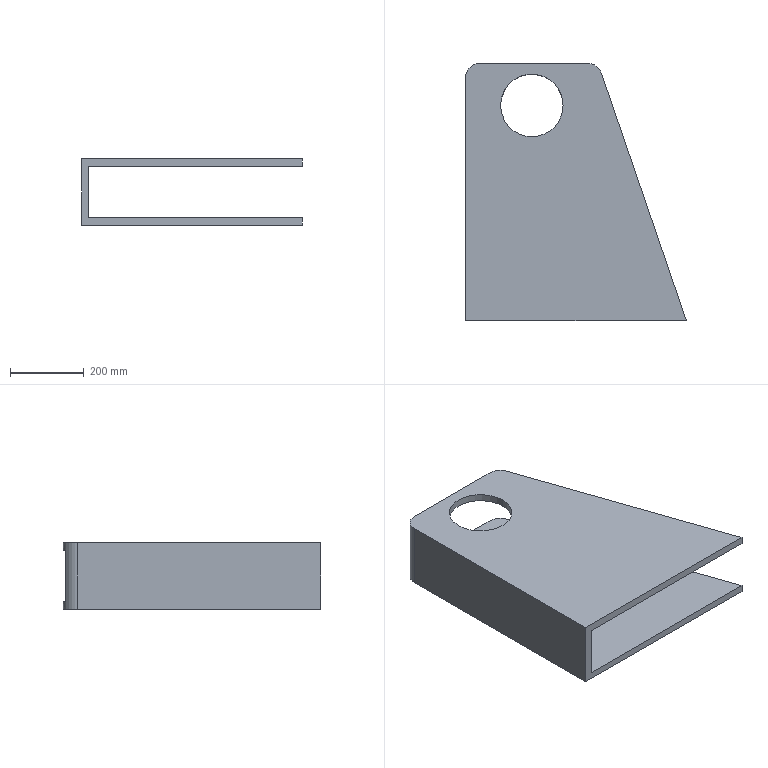Part | SolidWorks | features ICE 3, Fillet 2, Extrusion 1 | 1 solid | 18 faces | box 600 x 700 x 180 mm | volume 14429116 mm3 | plane 11 | cylinder 7 | commonest cylinder face diameters 170 x4 80 x3
STEP:
#1=CARTESIAN_POINT('',(95.,585.,-20.));
#2=VERTEX_POINT('',#1);
#3=CARTESIAN_POINT('',(265.,585.,-20.));
#4=VERTEX_POINT('',#3);
#5=CARTESIAN_POINT('',(180.,585.,-20.));
#6=DIRECTION('',(0.,0.,1.));
#7=DIRECTION('',(1.,0.,0.));
#8=AXIS2_PLACEMENT_3D('',#5,#6,#7);
#9=CIRCLE('',#8,85.);
#10=EDGE_CURVE('',#2,#4,#9,.T.);
#11=ORIENTED_EDGE('',*,*,#10,.F.);
#12=CARTESIAN_POINT('',(95.,585.,0.));
#13=VERTEX_POINT('',#12);
#14=CARTESIAN_POINT('',(95.,585.,-190.));
#15=DIRECTION('',(0.,0.,1.));
#16=VECTOR('',#15,1000.);
#17=LINE('',#14,#16);
#18=EDGE_CURVE('',#2,#13,#17,.T.);
#19=ORIENTED_EDGE('',*,*,#18,.T.);
#20=CARTESIAN_POINT('',(265.,585.,0.));
#21=VERTEX_POINT('',#20);
#22=CARTESIAN_POINT('',(180.,585.,0.));
#23=DIRECTION('',(0.,0.,1.));
#24=DIRECTION('',(1.,0.,0.));
#25=AXIS2_PLACEMENT_3D('',#22,#23,#24);
#26=CIRCLE('',#25,85.);
#27=EDGE_CURVE('',#13,#21,#26,.T.);
#28=ORIENTED_EDGE('',*,*,#27,.T.);
#29=CARTESIAN_POINT('',(265.,585.,-190.));
#30=DIRECTION('',(0.,0.,1.));
#31=VECTOR('',#30,1000.);
#32=LINE('',#29,#31);
#33=EDGE_CURVE('',#4,#21,#32,.T.);
#34=ORIENTED_EDGE('',*,*,#33,.F.);
#35=EDGE_LOOP('',(#11,#19,#28,#34));
#36=FACE_OUTER_BOUND('',#35,.T.);
#37=CARTESIAN_POINT('',(180.,585.,-190.));
#38=DIRECTION('',(0.,0.,1.));
#39=DIRECTION('',(1.,0.,0.));
#40=AXIS2_PLACEMENT_3D('',#37,#38,#39);
#41=CYLINDRICAL_SURFACE('',#40,85.);
#42=ADVANCED_FACE('',(#36),#41,.F.);
#43=CARTESIAN_POINT('',(95.,585.,-180.));
#44=VERTEX_POINT('',#43);
#45=CARTESIAN_POINT('',(265.,585.,-180.));
#46=VERTEX_POINT('',#45);
#47=CARTESIAN_POINT('',(180.,585.,-180.));
#48=DIRECTION('',(0.,0.,1.));
#49=DIRECTION('',(1.,0.,0.));
#50=AXIS2_PLACEMENT_3D('',#47,#48,#49);
#51=CIRCLE('',#50,85.);
#52=EDGE_CURVE('',#44,#46,#51,.T.);
#53=ORIENTED_EDGE('',*,*,#52,.F.);
#54=CARTESIAN_POINT('',(95.,585.,-160.));
#55=VERTEX_POINT('',#54);
#56=CARTESIAN_POINT('',(95.,585.,-190.));
#57=DIRECTION('',(0.,0.,1.));
#58=VECTOR('',#57,1000.);
#59=LINE('',#56,#58);
#60=EDGE_CURVE('',#44,#55,#59,.T.);
#61=ORIENTED_EDGE('',*,*,#60,.T.);
#62=CARTESIAN_POINT('',(265.,585.,-160.));
#63=VERTEX_POINT('',#62);
#64=CARTESIAN_POINT('',(180.,585.,-160.));
#65=DIRECTION('',(0.,0.,-1.));
#66=DIRECTION('',(-1.,0.,0.));
#67=AXIS2_PLACEMENT_3D('',#64,#65,#66);
#68=CIRCLE('',#67,85.);
#69=EDGE_CURVE('',#63,#55,#68,.T.);
#70=ORIENTED_EDGE('',*,*,#69,.F.);
#71=CARTESIAN_POINT('',(265.,585.,-190.));
#72=DIRECTION('',(0.,0.,1.));
#73=VECTOR('',#72,1000.);
#74=LINE('',#71,#73);
#75=EDGE_CURVE('',#46,#63,#74,.T.);
#76=ORIENTED_EDGE('',*,*,#75,.F.);
#77=EDGE_LOOP('',(#53,#61,#70,#76));
#78=FACE_OUTER_BOUND('',#77,.T.);
#79=CARTESIAN_POINT('',(180.,585.,-190.));
#80=DIRECTION('',(0.,0.,1.));
#81=DIRECTION('',(1.,0.,0.));
#82=AXIS2_PLACEMENT_3D('',#79,#80,#81);
#83=CYLINDRICAL_SURFACE('',#82,85.);
#84=ADVANCED_FACE('',(#78),#83,.F.);
#85=CARTESIAN_POINT('',(331.429,700.,-180.));
#86=VERTEX_POINT('',#85);
#87=CARTESIAN_POINT('',(40.,700.,-180.));
#88=VERTEX_POINT('',#87);
#89=CARTESIAN_POINT('',(0.,700.,-180.));
#90=DIRECTION('',(-1.,0.,0.));
#91=VECTOR('',#90,1000.);
#92=LINE('',#89,#91);
#93=EDGE_CURVE('',#86,#88,#92,.T.);
#94=ORIENTED_EDGE('',*,*,#93,.T.);
#95=CARTESIAN_POINT('',(40.,700.,-160.));
#96=VERTEX_POINT('',#95);
#97=CARTESIAN_POINT('',(40.,700.,0.));
#98=DIRECTION('',(0.,0.,1.));
#99=VECTOR('',#98,1000.);
#100=LINE('',#97,#99);
#101=EDGE_CURVE('',#88,#96,#100,.T.);
#102=ORIENTED_EDGE('',*,*,#101,.T.);
#103=CARTESIAN_POINT('',(331.429,700.,-160.));
#104=VERTEX_POINT('',#103);
#105=CARTESIAN_POINT('',(360.,700.,-160.));
#106=DIRECTION('',(1.,0.,0.));
#107=VECTOR('',#106,1000.);
#108=LINE('',#105,#107);
#109=EDGE_CURVE('',#96,#104,#108,.T.);
#110=ORIENTED_EDGE('',*,*,#109,.T.);
#111=CARTESIAN_POINT('',(331.429,700.,-180.));
#112=DIRECTION('',(0.,0.,-1.));
#113=VECTOR('',#112,1000.);
#114=LINE('',#111,#113);
#115=EDGE_CURVE('',#104,#86,#114,.T.);
#116=ORIENTED_EDGE('',*,*,#115,.T.);
#117=EDGE_LOOP('',(#94,#102,#110,#116));
#118=FACE_OUTER_BOUND('',#117,.T.);
#119=CARTESIAN_POINT('',(0.,700.,0.));
#120=DIRECTION('',(0.,-1.,0.));
#121=DIRECTION('',(0.,0.,-1.));
#122=AXIS2_PLACEMENT_3D('',#119,#120,#121);
#123=PLANE('',#122);
#124=ADVANCED_FACE('',(#118),#123,.F.);
#125=CARTESIAN_POINT('',(180.,585.,0.));
#126=DIRECTION('',(0.,0.,1.));
#127=DIRECTION('',(1.,0.,0.));
#128=AXIS2_PLACEMENT_3D('',#125,#126,#127);
#129=CIRCLE('',#128,85.);
#130=EDGE_CURVE('',#21,#13,#129,.T.);
#131=ORIENTED_EDGE('',*,*,#130,.F.);
#132=ORIENTED_EDGE('',*,*,#27,.F.);
#133=EDGE_LOOP('',(#131,#132));
#134=FACE_BOUND('',#133,.T.);
#135=CARTESIAN_POINT('',(40.,700.,0.));
#136=VERTEX_POINT('',#135);
#137=CARTESIAN_POINT('',(331.429,700.,0.));
#138=VERTEX_POINT('',#137);
#139=CARTESIAN_POINT('',(360.,700.,0.));
#140=DIRECTION('',(1.,0.,0.));
#141=VECTOR('',#140,1000.);
#142=LINE('',#139,#141);
#143=EDGE_CURVE('',#136,#138,#142,.T.);
#144=ORIENTED_EDGE('',*,*,#143,.F.);
#145=CARTESIAN_POINT('',(0.,660.,0.));
#146=VERTEX_POINT('',#145);
#147=CARTESIAN_POINT('',(40.,660.,0.));
#148=DIRECTION('',(0.,0.,1.));
#149=DIRECTION('',(-1.,0.,0.));
#150=AXIS2_PLACEMENT_3D('',#147,#148,#149);
#151=CIRCLE('',#150,40.);
#152=EDGE_CURVE('',#136,#146,#151,.T.);
#153=ORIENTED_EDGE('',*,*,#152,.T.);
#154=CARTESIAN_POINT('',(0.,0.,0.));
#155=VERTEX_POINT('',#154);
#156=CARTESIAN_POINT('',(0.,700.,0.));
#157=DIRECTION('',(0.,-1.,0.));
#158=VECTOR('',#157,1000.);
#159=LINE('',#156,#158);
#160=EDGE_CURVE('',#146,#155,#159,.T.);
#161=ORIENTED_EDGE('',*,*,#160,.T.);
#162=CARTESIAN_POINT('',(600.,0.,0.));
#163=VERTEX_POINT('',#162);
#164=CARTESIAN_POINT('',(360.,0.,0.));
#165=DIRECTION('',(1.,0.,0.));
#166=VECTOR('',#165,1000.);
#167=LINE('',#164,#166);
#168=EDGE_CURVE('',#155,#163,#167,.T.);
#169=ORIENTED_EDGE('',*,*,#168,.T.);
#170=CARTESIAN_POINT('',(369.266,672.973,0.));
#171=VERTEX_POINT('',#170);
#172=CARTESIAN_POINT('',(360.,700.,0.));
#173=DIRECTION('',(-0.3243,0.9459,0.));
#174=VECTOR('',#173,1000.);
#175=LINE('',#172,#174);
#176=EDGE_CURVE('',#163,#171,#175,.T.);
#177=ORIENTED_EDGE('',*,*,#176,.T.);
#178=CARTESIAN_POINT('',(331.429,660.,0.));
#179=DIRECTION('',(0.,0.,1.));
#180=DIRECTION('',(-1.,0.,0.));
#181=AXIS2_PLACEMENT_3D('',#178,#179,#180);
#182=CIRCLE('',#181,40.);
#183=EDGE_CURVE('',#171,#138,#182,.T.);
#184=ORIENTED_EDGE('',*,*,#183,.T.);
#185=EDGE_LOOP('',(#144,#153,#161,#169,#177,#184));
#186=FACE_OUTER_BOUND('',#185,.T.);
#187=CARTESIAN_POINT('',(360.,700.,0.));
#188=DIRECTION('',(0.,0.,-1.));
#189=DIRECTION('',(-1.,0.,0.));
#190=AXIS2_PLACEMENT_3D('',#187,#188,#189);
#191=PLANE('',#190);
#192=ADVANCED_FACE('',(#134,#186),#191,.F.);
#193=CARTESIAN_POINT('',(180.,585.,-20.));
#194=DIRECTION('',(0.,0.,1.));
#195=DIRECTION('',(1.,0.,0.));
#196=AXIS2_PLACEMENT_3D('',#193,#194,#195);
#197=CIRCLE('',#196,85.);
#198=EDGE_CURVE('',#4,#2,#197,.T.);
#199=ORIENTED_EDGE('',*,*,#198,.T.);
#200=ORIENTED_EDGE('',*,*,#10,.T.);
#201=EDGE_LOOP('',(#199,#200));
#202=FACE_BOUND('',#201,.T.);
#203=CARTESIAN_POINT('',(20.,694.641,-20.));
#204=VERTEX_POINT('',#203);
#205=CARTESIAN_POINT('',(20.,0.,-20.));
#206=VERTEX_POINT('',#205);
#207=CARTESIAN_POINT('',(20.,700.,-20.));
#208=DIRECTION('',(0.,-1.,0.));
#209=VECTOR('',#208,1000.);
#210=LINE('',#207,#209);
#211=EDGE_CURVE('',#204,#206,#210,.T.);
#212=ORIENTED_EDGE('',*,*,#211,.F.);
#213=CARTESIAN_POINT('',(40.,700.,-20.));
#214=VERTEX_POINT('',#213);
#215=CARTESIAN_POINT('',(40.,660.,-20.));
#216=DIRECTION('',(0.,0.,-1.));
#217=DIRECTION('',(1.,0.,0.));
#218=AXIS2_PLACEMENT_3D('',#215,#216,#217);
#219=CIRCLE('',#218,40.);
#220=EDGE_CURVE('',#204,#214,#219,.T.);
#221=ORIENTED_EDGE('',*,*,#220,.T.);
#222=CARTESIAN_POINT('',(331.429,700.,-20.));
#223=VERTEX_POINT('',#222);
#224=CARTESIAN_POINT('',(20.,700.,-20.));
#225=DIRECTION('',(-1.,0.,0.));
#226=VECTOR('',#225,1000.);
#227=LINE('',#224,#226);
#228=EDGE_CURVE('',#223,#214,#227,.T.);
#229=ORIENTED_EDGE('',*,*,#228,.F.);
#230=CARTESIAN_POINT('',(369.266,672.973,-20.));
#231=VERTEX_POINT('',#230);
#232=CARTESIAN_POINT('',(331.429,660.,-20.));
#233=DIRECTION('',(0.,0.,-1.));
#234=DIRECTION('',(1.,0.,0.));
#235=AXIS2_PLACEMENT_3D('',#232,#233,#234);
#236=CIRCLE('',#235,40.);
#237=EDGE_CURVE('',#223,#231,#236,.T.);
#238=ORIENTED_EDGE('',*,*,#237,.T.);
#239=CARTESIAN_POINT('',(600.,0.,-20.));
#240=VERTEX_POINT('',#239);
#241=CARTESIAN_POINT('',(360.,700.,-20.));
#242=DIRECTION('',(-0.3243,0.9459,0.));
#243=VECTOR('',#242,1000.);
#244=LINE('',#241,#243);
#245=EDGE_CURVE('',#240,#231,#244,.T.);
#246=ORIENTED_EDGE('',*,*,#245,.F.);
#247=CARTESIAN_POINT('',(20.,0.,-20.));
#248=DIRECTION('',(-1.,0.,0.));
#249=VECTOR('',#248,1000.);
#250=LINE('',#247,#249);
#251=EDGE_CURVE('',#240,#206,#250,.T.);
#252=ORIENTED_EDGE('',*,*,#251,.T.);
#253=EDGE_LOOP('',(#212,#221,#229,#238,#246,#252));
#254=FACE_OUTER_BOUND('',#253,.T.);
#255=CARTESIAN_POINT('',(20.,700.,-20.));
#256=DIRECTION('',(0.,0.,1.));
#257=DIRECTION('',(1.,0.,0.));
#258=AXIS2_PLACEMENT_3D('',#255,#256,#257);
#259=PLANE('',#258);
#260=ADVANCED_FACE('',(#202,#254),#259,.F.);
#261=CARTESIAN_POINT('',(20.,694.641,-160.));
#262=VERTEX_POINT('',#261);
#263=CARTESIAN_POINT('',(20.,0.,-160.));
#264=VERTEX_POINT('',#263);
#265=CARTESIAN_POINT('',(20.,700.,-160.));
#266=DIRECTION('',(0.,-1.,0.));
#267=VECTOR('',#266,1000.);
#268=LINE('',#265,#267);
#269=EDGE_CURVE('',#262,#264,#268,.T.);
#270=ORIENTED_EDGE('',*,*,#269,.F.);
#271=CARTESIAN_POINT('',(20.,694.641,-160.));
#272=DIRECTION('',(0.,0.,1.));
#273=VECTOR('',#272,1000.);
#274=LINE('',#271,#273);
#275=EDGE_CURVE('',#262,#204,#274,.T.);
#276=ORIENTED_EDGE('',*,*,#275,.T.);
#277=ORIENTED_EDGE('',*,*,#211,.T.);
#278=CARTESIAN_POINT('',(20.,0.,-160.));
#279=DIRECTION('',(0.,0.,-1.));
#280=VECTOR('',#279,1000.);
#281=LINE('',#278,#280);
#282=EDGE_CURVE('',#206,#264,#281,.T.);
#283=ORIENTED_EDGE('',*,*,#282,.T.);
#284=EDGE_LOOP('',(#270,#276,#277,#283));
#285=FACE_OUTER_BOUND('',#284,.T.);
#286=CARTESIAN_POINT('',(20.,700.,-160.));
#287=DIRECTION('',(-1.,0.,0.));
#288=DIRECTION('',(0.,0.,1.));
#289=AXIS2_PLACEMENT_3D('',#286,#287,#288);
#290=PLANE('',#289);
#291=ADVANCED_FACE('',(#285),#290,.F.);
#292=ORIENTED_EDGE('',*,*,#69,.T.);
#293=CARTESIAN_POINT('',(180.,585.,-160.));
#294=DIRECTION('',(0.,0.,-1.));
#295=DIRECTION('',(-1.,0.,0.));
#296=AXIS2_PLACEMENT_3D('',#293,#294,#295);
#297=CIRCLE('',#296,85.);
#298=EDGE_CURVE('',#55,#63,#297,.T.);
#299=ORIENTED_EDGE('',*,*,#298,.T.);
#300=EDGE_LOOP('',(#292,#299));
#301=FACE_BOUND('',#300,.T.);
#302=ORIENTED_EDGE('',*,*,#109,.F.);
#303=CARTESIAN_POINT('',(40.,660.,-160.));
#304=DIRECTION('',(0.,0.,1.));
#305=DIRECTION('',(-1.,0.,0.));
#306=AXIS2_PLACEMENT_3D('',#303,#304,#305);
#307=CIRCLE('',#306,40.);
#308=EDGE_CURVE('',#96,#262,#307,.T.);
#309=ORIENTED_EDGE('',*,*,#308,.T.);
#310=ORIENTED_EDGE('',*,*,#269,.T.);
#311=CARTESIAN_POINT('',(600.,0.,-160.));
#312=VERTEX_POINT('',#311);
#313=CARTESIAN_POINT('',(360.,0.,-160.));
#314=DIRECTION('',(1.,0.,0.));
#315=VECTOR('',#314,1000.);
#316=LINE('',#313,#315);
#317=EDGE_CURVE('',#264,#312,#316,.T.);
#318=ORIENTED_EDGE('',*,*,#317,.T.);
#319=CARTESIAN_POINT('',(369.266,672.973,-160.));
#320=VERTEX_POINT('',#319);
#321=CARTESIAN_POINT('',(600.,0.,-160.));
#322=DIRECTION('',(0.3243,-0.9459,0.));
#323=VECTOR('',#322,1000.);
#324=LINE('',#321,#323);
#325=EDGE_CURVE('',#320,#312,#324,.T.);
#326=ORIENTED_EDGE('',*,*,#325,.F.);
#327=CARTESIAN_POINT('',(331.429,660.,-160.));
#328=DIRECTION('',(0.,0.,1.));
#329=DIRECTION('',(-1.,0.,0.));
#330=AXIS2_PLACEMENT_3D('',#327,#328,#329);
#331=CIRCLE('',#330,40.);
#332=EDGE_CURVE('',#320,#104,#331,.T.);
#333=ORIENTED_EDGE('',*,*,#332,.T.);
#334=EDGE_LOOP('',(#302,#309,#310,#318,#326,#333));
#335=FACE_OUTER_BOUND('',#334,.T.);
#336=CARTESIAN_POINT('',(360.,700.,-160.));
#337=DIRECTION('',(0.,0.,-1.));
#338=DIRECTION('',(-1.,0.,0.));
#339=AXIS2_PLACEMENT_3D('',#336,#337,#338);
#340=PLANE('',#339);
#341=ADVANCED_FACE('',(#301,#335),#340,.F.);
#342=CARTESIAN_POINT('',(180.,585.,-180.));
#343=DIRECTION('',(0.,0.,1.));
#344=DIRECTION('',(1.,0.,0.));
#345=AXIS2_PLACEMENT_3D('',#342,#343,#344);
#346=CIRCLE('',#345,85.);
#347=EDGE_CURVE('',#46,#44,#346,.T.);
#348=ORIENTED_EDGE('',*,*,#347,.T.);
#349=ORIENTED_EDGE('',*,*,#52,.T.);
#350=EDGE_LOOP('',(#348,#349));
#351=FACE_BOUND('',#350,.T.);
#352=CARTESIAN_POINT('',(0.,660.,-180.));
#353=VERTEX_POINT('',#352);
#354=CARTESIAN_POINT('',(0.,0.,-180.));
#355=VERTEX_POINT('',#354);
#356=CARTESIAN_POINT('',(0.,700.,-180.));
#357=DIRECTION('',(0.,-1.,0.));
#358=VECTOR('',#357,1000.);
#359=LINE('',#356,#358);
#360=EDGE_CURVE('',#353,#355,#359,.T.);
#361=ORIENTED_EDGE('',*,*,#360,.F.);
#362=CARTESIAN_POINT('',(40.,660.,-180.));
#363=DIRECTION('',(0.,0.,-1.));
#364=DIRECTION('',(1.,0.,0.));
#365=AXIS2_PLACEMENT_3D('',#362,#363,#364);
#366=CIRCLE('',#365,40.);
#367=EDGE_CURVE('',#353,#88,#366,.T.);
#368=ORIENTED_EDGE('',*,*,#367,.T.);
#369=ORIENTED_EDGE('',*,*,#93,.F.);
#370=CARTESIAN_POINT('',(369.266,672.973,-180.));
#371=VERTEX_POINT('',#370);
#372=CARTESIAN_POINT('',(331.429,660.,-180.));
#373=DIRECTION('',(0.,0.,-1.));
#374=DIRECTION('',(1.,0.,0.));
#375=AXIS2_PLACEMENT_3D('',#372,#373,#374);
#376=CIRCLE('',#375,40.);
#377=EDGE_CURVE('',#86,#371,#376,.T.);
#378=ORIENTED_EDGE('',*,*,#377,.T.);
#379=CARTESIAN_POINT('',(600.,0.,-180.));
#380=VERTEX_POINT('',#379);
#381=CARTESIAN_POINT('',(600.,0.,-180.));
#382=DIRECTION('',(0.3243,-0.9459,0.));
#383=VECTOR('',#382,1000.);
#384=LINE('',#381,#383);
#385=EDGE_CURVE('',#371,#380,#384,.T.);
#386=ORIENTED_EDGE('',*,*,#385,.T.);
#387=CARTESIAN_POINT('',(0.,0.,-180.));
#388=DIRECTION('',(-1.,0.,0.));
#389=VECTOR('',#388,1000.);
#390=LINE('',#387,#389);
#391=EDGE_CURVE('',#380,#355,#390,.T.);
#392=ORIENTED_EDGE('',*,*,#391,.T.);
#393=EDGE_LOOP('',(#361,#368,#369,#378,#386,#392));
#394=FACE_OUTER_BOUND('',#393,.T.);
#395=CARTESIAN_POINT('',(0.,700.,-180.));
#396=DIRECTION('',(0.,0.,1.));
#397=DIRECTION('',(1.,0.,0.));
#398=AXIS2_PLACEMENT_3D('',#395,#396,#397);
#399=PLANE('',#398);
#400=ADVANCED_FACE('',(#351,#394),#399,.F.);
#401=ORIENTED_EDGE('',*,*,#160,.F.);
#402=CARTESIAN_POINT('',(0.,660.,0.));
#403=DIRECTION('',(0.,0.,-1.));
#404=VECTOR('',#403,1000.);
#405=LINE('',#402,#404);
#406=EDGE_CURVE('',#146,#353,#405,.T.);
#407=ORIENTED_EDGE('',*,*,#406,.T.);
#408=ORIENTED_EDGE('',*,*,#360,.T.);
#409=CARTESIAN_POINT('',(0.,0.,0.));
#410=DIRECTION('',(0.,0.,1.));
#411=VECTOR('',#410,1000.);
#412=LINE('',#409,#411);
#413=EDGE_CURVE('',#355,#155,#412,.T.);
#414=ORIENTED_EDGE('',*,*,#413,.T.);
#415=EDGE_LOOP('',(#401,#407,#408,#414));
#416=FACE_OUTER_BOUND('',#415,.T.);
#417=CARTESIAN_POINT('',(0.,700.,0.));
#418=DIRECTION('',(1.,0.,0.));
#419=DIRECTION('',(0.,0.,-1.));
#420=AXIS2_PLACEMENT_3D('',#417,#418,#419);
#421=PLANE('',#420);
#422=ADVANCED_FACE('',(#416),#421,.F.);
#423=ORIENTED_EDGE('',*,*,#228,.T.);
#424=CARTESIAN_POINT('',(40.,700.,0.));
#425=DIRECTION('',(0.,0.,1.));
#426=VECTOR('',#425,1000.);
#427=LINE('',#424,#426);
#428=EDGE_CURVE('',#214,#136,#427,.T.);
#429=ORIENTED_EDGE('',*,*,#428,.T.);
#430=ORIENTED_EDGE('',*,*,#143,.T.);
#431=CARTESIAN_POINT('',(331.429,700.,-20.));
#432=DIRECTION('',(0.,0.,-1.));
#433=VECTOR('',#432,1000.);
#434=LINE('',#431,#433);
#435=EDGE_CURVE('',#138,#223,#434,.T.);
#436=ORIENTED_EDGE('',*,*,#435,.T.);
#437=EDGE_LOOP('',(#423,#429,#430,#436));
#438=FACE_OUTER_BOUND('',#437,.T.);
#439=CARTESIAN_POINT('',(0.,700.,0.));
#440=DIRECTION('',(0.,-1.,0.));
#441=DIRECTION('',(0.,0.,-1.));
#442=AXIS2_PLACEMENT_3D('',#439,#440,#441);
#443=PLANE('',#442);
#444=ADVANCED_FACE('',(#438),#443,.F.);
#445=ORIENTED_EDGE('',*,*,#168,.F.);
#446=ORIENTED_EDGE('',*,*,#413,.F.);
#447=ORIENTED_EDGE('',*,*,#391,.F.);
#448=CARTESIAN_POINT('',(600.,0.,-160.));
#449=DIRECTION('',(0.,0.,-1.));
#450=VECTOR('',#449,1000.);
#451=LINE('',#448,#450);
#452=EDGE_CURVE('',#312,#380,#451,.T.);
#453=ORIENTED_EDGE('',*,*,#452,.F.);
#454=ORIENTED_EDGE('',*,*,#317,.F.);
#455=ORIENTED_EDGE('',*,*,#282,.F.);
#456=ORIENTED_EDGE('',*,*,#251,.F.);
#457=CARTESIAN_POINT('',(600.,0.,-20.));
#458=DIRECTION('',(0.,0.,1.));
#459=VECTOR('',#458,1000.);
#460=LINE('',#457,#459);
#461=EDGE_CURVE('',#240,#163,#460,.T.);
#462=ORIENTED_EDGE('',*,*,#461,.T.);
#463=EDGE_LOOP('',(#445,#446,#447,#453,#454,#455,#456,#462));
#464=FACE_OUTER_BOUND('',#463,.T.);
#465=CARTESIAN_POINT('',(0.,0.,0.));
#466=DIRECTION('',(0.,-1.,0.));
#467=DIRECTION('',(0.,0.,-1.));
#468=AXIS2_PLACEMENT_3D('',#465,#466,#467);
#469=PLANE('',#468);
#470=ADVANCED_FACE('',(#464),#469,.T.);
#471=ORIENTED_EDGE('',*,*,#60,.F.);
#472=ORIENTED_EDGE('',*,*,#347,.F.);
#473=ORIENTED_EDGE('',*,*,#75,.T.);
#474=ORIENTED_EDGE('',*,*,#298,.F.);
#475=EDGE_LOOP('',(#471,#472,#473,#474));
#476=FACE_OUTER_BOUND('',#475,.T.);
#477=CARTESIAN_POINT('',(180.,585.,-190.));
#478=DIRECTION('',(0.,0.,1.));
#479=DIRECTION('',(1.,0.,0.));
#480=AXIS2_PLACEMENT_3D('',#477,#478,#479);
#481=CYLINDRICAL_SURFACE('',#480,85.);
#482=ADVANCED_FACE('',(#476),#481,.F.);
#483=ORIENTED_EDGE('',*,*,#18,.F.);
#484=ORIENTED_EDGE('',*,*,#198,.F.);
#485=ORIENTED_EDGE('',*,*,#33,.T.);
#486=ORIENTED_EDGE('',*,*,#130,.T.);
#487=EDGE_LOOP('',(#483,#484,#485,#486));
#488=FACE_OUTER_BOUND('',#487,.T.);
#489=CARTESIAN_POINT('',(180.,585.,-190.));
#490=DIRECTION('',(0.,0.,1.));
#491=DIRECTION('',(1.,0.,0.));
#492=AXIS2_PLACEMENT_3D('',#489,#490,#491);
#493=CYLINDRICAL_SURFACE('',#492,85.);
#494=ADVANCED_FACE('',(#488),#493,.F.);
#495=ORIENTED_EDGE('',*,*,#245,.T.);
#496=CARTESIAN_POINT('',(369.266,672.973,0.));
#497=DIRECTION('',(0.,0.,1.));
#498=VECTOR('',#497,1000.);
#499=LINE('',#496,#498);
#500=EDGE_CURVE('',#231,#171,#499,.T.);
#501=ORIENTED_EDGE('',*,*,#500,.T.);
#502=ORIENTED_EDGE('',*,*,#176,.F.);
#503=ORIENTED_EDGE('',*,*,#461,.F.);
#504=EDGE_LOOP('',(#495,#501,#502,#503));
#505=FACE_OUTER_BOUND('',#504,.T.);
#506=CARTESIAN_POINT('',(360.,700.,-20.));
#507=DIRECTION('',(0.9459,0.3243,0.));
#508=DIRECTION('',(-0.3243,0.9459,0.));
#509=AXIS2_PLACEMENT_3D('',#506,#507,#508);
#510=PLANE('',#509);
#511=ADVANCED_FACE('',(#505),#510,.T.);
#512=ORIENTED_EDGE('',*,*,#385,.F.);
#513=CARTESIAN_POINT('',(369.266,672.973,-160.));
#514=DIRECTION('',(0.,0.,1.));
#515=VECTOR('',#514,1000.);
#516=LINE('',#513,#515);
#517=EDGE_CURVE('',#371,#320,#516,.T.);
#518=ORIENTED_EDGE('',*,*,#517,.T.);
#519=ORIENTED_EDGE('',*,*,#325,.T.);
#520=ORIENTED_EDGE('',*,*,#452,.T.);
#521=EDGE_LOOP('',(#512,#518,#519,#520));
#522=FACE_OUTER_BOUND('',#521,.T.);
#523=CARTESIAN_POINT('',(600.,0.,-160.));
#524=DIRECTION('',(0.9459,0.3243,0.));
#525=DIRECTION('',(-0.3243,0.9459,0.));
#526=AXIS2_PLACEMENT_3D('',#523,#524,#525);
#527=PLANE('',#526);
#528=ADVANCED_FACE('',(#522),#527,.T.);
#529=ORIENTED_EDGE('',*,*,#332,.F.);
#530=ORIENTED_EDGE('',*,*,#517,.F.);
#531=ORIENTED_EDGE('',*,*,#377,.F.);
#532=ORIENTED_EDGE('',*,*,#115,.F.);
#533=EDGE_LOOP('',(#529,#530,#531,#532));
#534=FACE_OUTER_BOUND('',#533,.T.);
#535=CARTESIAN_POINT('',(331.429,660.,0.));
#536=DIRECTION('',(0.,0.,1.));
#537=DIRECTION('',(1.,0.,0.));
#538=AXIS2_PLACEMENT_3D('',#535,#536,#537);
#539=CYLINDRICAL_SURFACE('',#538,40.);
#540=ADVANCED_FACE('',(#534),#539,.T.);
#541=ORIENTED_EDGE('',*,*,#183,.F.);
#542=ORIENTED_EDGE('',*,*,#500,.F.);
#543=ORIENTED_EDGE('',*,*,#237,.F.);
#544=ORIENTED_EDGE('',*,*,#435,.F.);
#545=EDGE_LOOP('',(#541,#542,#543,#544));
#546=FACE_OUTER_BOUND('',#545,.T.);
#547=CARTESIAN_POINT('',(331.429,660.,0.));
#548=DIRECTION('',(0.,0.,1.));
#549=DIRECTION('',(1.,0.,0.));
#550=AXIS2_PLACEMENT_3D('',#547,#548,#549);
#551=CYLINDRICAL_SURFACE('',#550,40.);
#552=ADVANCED_FACE('',(#546),#551,.T.);
#553=ORIENTED_EDGE('',*,*,#367,.F.);
#554=ORIENTED_EDGE('',*,*,#406,.F.);
#555=ORIENTED_EDGE('',*,*,#152,.F.);
#556=ORIENTED_EDGE('',*,*,#428,.F.);
#557=ORIENTED_EDGE('',*,*,#220,.F.);
#558=ORIENTED_EDGE('',*,*,#275,.F.);
#559=ORIENTED_EDGE('',*,*,#308,.F.);
#560=ORIENTED_EDGE('',*,*,#101,.F.);
#561=EDGE_LOOP('',(#553,#554,#555,#556,#557,#558,#559,#560));
#562=FACE_OUTER_BOUND('',#561,.T.);
#563=CARTESIAN_POINT('',(40.,660.,0.));
#564=DIRECTION('',(0.,0.,1.));
#565=DIRECTION('',(1.,0.,0.));
#566=AXIS2_PLACEMENT_3D('',#563,#564,#565);
#567=CYLINDRICAL_SURFACE('',#566,40.);
#568=ADVANCED_FACE('',(#562),#567,.T.);
#569=CLOSED_SHELL('',(#42,#84,#124,#192,#260,#291,#341,#400,#422,#444,#470,#482,#494,#511,#528,#540,#552,#568));
#570=MANIFOLD_SOLID_BREP('',#569);
#571=CARTESIAN_POINT('',(0.,0.,0.));
#572=DIRECTION('',(0.,0.,1.));
#573=DIRECTION('',(1.,0.,0.));
#574=AXIS2_PLACEMENT_3D('',#571,#572,#573);
#575=(LENGTH_UNIT()NAMED_UNIT(*)SI_UNIT(.MILLI.,.METRE.));
#576=UNCERTAINTY_MEASURE_WITH_UNIT(LENGTH_MEASURE(0.00001),#575,'','');
#577=(NAMED_UNIT(*)PLANE_ANGLE_UNIT()SI_UNIT($,.RADIAN.));
#578=(NAMED_UNIT(*)SI_UNIT($,.STERADIAN.)SOLID_ANGLE_UNIT());
#579=(GEOMETRIC_REPRESENTATION_CONTEXT(3)GLOBAL_UNCERTAINTY_ASSIGNED_CONTEXT((#576))GLOBAL_UNIT_ASSIGNED_CONTEXT((#575,#577,#578))REPRESENTATION_CONTEXT('',''));
#580=ADVANCED_BREP_SHAPE_REPRESENTATION('',(#570,#574),#579);